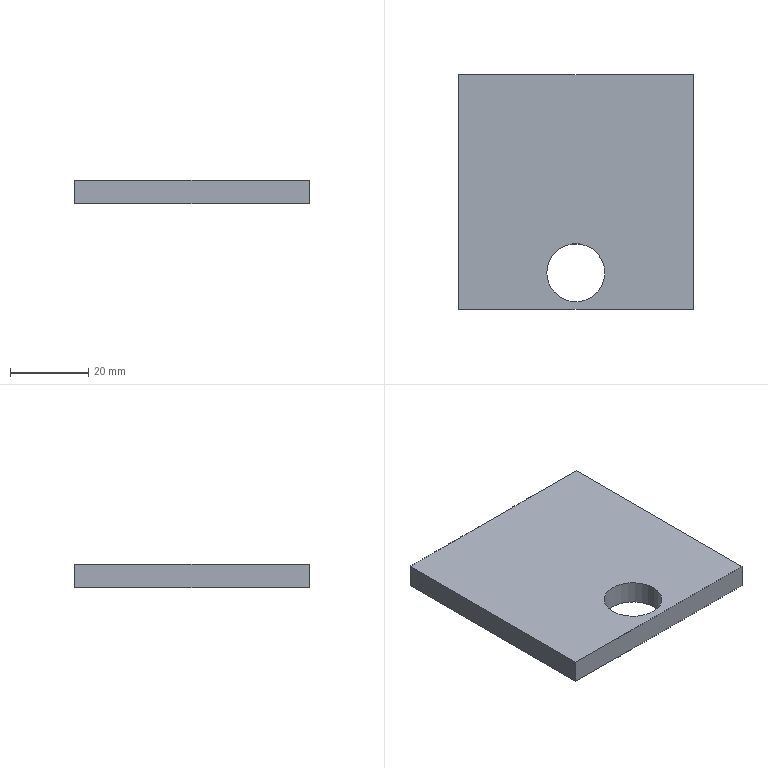Part | NX | features 凸台-拉伸21[4] 2 | 1 solid | 8 faces | box 60 x 60 x 6 mm | volume 20564 mm3 | plane 6 | cylinder 2 | commonest cylinder face diameters 14.829 x2
STEP:
#1=CARTESIAN_POINT('',(2895.533,-50.65,291.015));
#2=VERTEX_POINT('',#1);
#3=CARTESIAN_POINT('',(2895.533,-50.65,297.015));
#4=VERTEX_POINT('',#3);
#5=CARTESIAN_POINT('',(2895.533,-50.65,291.015));
#6=DIRECTION('',(0.,0.,1.));
#7=VECTOR('',#6,1000.);
#8=LINE('',#5,#7);
#9=EDGE_CURVE('',#2,#4,#8,.T.);
#10=ORIENTED_EDGE('',*,*,#9,.F.);
#11=CARTESIAN_POINT('',(2910.361,-50.65,291.015));
#12=VERTEX_POINT('',#11);
#13=CARTESIAN_POINT('',(2902.947,-50.65,291.015));
#14=DIRECTION('',(0.,0.,-1.));
#15=DIRECTION('',(-1.,0.,0.));
#16=AXIS2_PLACEMENT_3D('',#13,#14,#15);
#17=CIRCLE('',#16,7.414);
#18=EDGE_CURVE('',#2,#12,#17,.T.);
#19=ORIENTED_EDGE('',*,*,#18,.T.);
#20=CARTESIAN_POINT('',(2910.361,-50.65,297.015));
#21=VERTEX_POINT('',#20);
#22=CARTESIAN_POINT('',(2910.361,-50.65,291.015));
#23=DIRECTION('',(0.,0.,1.));
#24=VECTOR('',#23,1000.);
#25=LINE('',#22,#24);
#26=EDGE_CURVE('',#21,#12,#25,.F.);
#27=ORIENTED_EDGE('',*,*,#26,.F.);
#28=CARTESIAN_POINT('',(2902.947,-50.65,297.015));
#29=DIRECTION('',(0.,0.,-1.));
#30=DIRECTION('',(-1.,0.,0.));
#31=AXIS2_PLACEMENT_3D('',#28,#29,#30);
#32=CIRCLE('',#31,7.414);
#33=EDGE_CURVE('',#4,#21,#32,.T.);
#34=ORIENTED_EDGE('',*,*,#33,.F.);
#35=EDGE_LOOP('',(#10,#19,#27,#34));
#36=FACE_BOUND('',#35,.T.);
#37=CARTESIAN_POINT('',(2902.947,-50.65,291.015));
#38=DIRECTION('',(0.,0.,1.));
#39=DIRECTION('',(1.,0.,0.));
#40=AXIS2_PLACEMENT_3D('',#37,#38,#39);
#41=CYLINDRICAL_SURFACE('',#40,7.414);
#42=ADVANCED_FACE('',(#36),#41,.F.);
#43=CARTESIAN_POINT('',(2933.,-60.,297.015));
#44=VERTEX_POINT('',#43);
#45=CARTESIAN_POINT('',(2873.,-60.,297.015));
#46=VERTEX_POINT('',#45);
#47=CARTESIAN_POINT('',(2873.,-60.,297.015));
#48=DIRECTION('',(-1.,0.,0.));
#49=VECTOR('',#48,1000.);
#50=LINE('',#47,#49);
#51=EDGE_CURVE('',#44,#46,#50,.T.);
#52=ORIENTED_EDGE('',*,*,#51,.T.);
#53=CARTESIAN_POINT('',(2873.,-60.,291.015));
#54=VERTEX_POINT('',#53);
#55=CARTESIAN_POINT('',(2873.,-60.,291.015));
#56=DIRECTION('',(0.,0.,1.));
#57=VECTOR('',#56,1000.);
#58=LINE('',#55,#57);
#59=EDGE_CURVE('',#54,#46,#58,.T.);
#60=ORIENTED_EDGE('',*,*,#59,.F.);
#61=CARTESIAN_POINT('',(2933.,-60.,291.015));
#62=VERTEX_POINT('',#61);
#63=CARTESIAN_POINT('',(2873.,-60.,291.015));
#64=DIRECTION('',(-1.,0.,0.));
#65=VECTOR('',#64,1000.);
#66=LINE('',#63,#65);
#67=EDGE_CURVE('',#62,#54,#66,.T.);
#68=ORIENTED_EDGE('',*,*,#67,.F.);
#69=CARTESIAN_POINT('',(2933.,-60.,291.015));
#70=DIRECTION('',(0.,0.,1.));
#71=VECTOR('',#70,1000.);
#72=LINE('',#69,#71);
#73=EDGE_CURVE('',#62,#44,#72,.T.);
#74=ORIENTED_EDGE('',*,*,#73,.T.);
#75=EDGE_LOOP('',(#52,#60,#68,#74));
#76=FACE_BOUND('',#75,.T.);
#77=CARTESIAN_POINT('',(2873.,-60.,291.015));
#78=DIRECTION('',(0.,1.,0.));
#79=DIRECTION('',(-1.,0.,0.));
#80=AXIS2_PLACEMENT_3D('',#77,#78,#79);
#81=PLANE('',#80);
#82=ADVANCED_FACE('',(#76),#81,.F.);
#83=CARTESIAN_POINT('',(2933.,0.,297.015));
#84=VERTEX_POINT('',#83);
#85=CARTESIAN_POINT('',(2933.,0.,297.015));
#86=DIRECTION('',(0.,-1.,0.));
#87=VECTOR('',#86,1000.);
#88=LINE('',#85,#87);
#89=EDGE_CURVE('',#84,#44,#88,.T.);
#90=ORIENTED_EDGE('',*,*,#89,.T.);
#91=ORIENTED_EDGE('',*,*,#73,.F.);
#92=CARTESIAN_POINT('',(2933.,0.,291.015));
#93=VERTEX_POINT('',#92);
#94=CARTESIAN_POINT('',(2933.,0.,291.015));
#95=DIRECTION('',(0.,-1.,0.));
#96=VECTOR('',#95,1000.);
#97=LINE('',#94,#96);
#98=EDGE_CURVE('',#93,#62,#97,.T.);
#99=ORIENTED_EDGE('',*,*,#98,.F.);
#100=CARTESIAN_POINT('',(2933.,0.,291.015));
#101=DIRECTION('',(0.,0.,1.));
#102=VECTOR('',#101,1000.);
#103=LINE('',#100,#102);
#104=EDGE_CURVE('',#93,#84,#103,.T.);
#105=ORIENTED_EDGE('',*,*,#104,.T.);
#106=EDGE_LOOP('',(#90,#91,#99,#105));
#107=FACE_BOUND('',#106,.T.);
#108=CARTESIAN_POINT('',(2933.,0.,291.015));
#109=DIRECTION('',(-1.,0.,0.));
#110=DIRECTION('',(0.,-1.,0.));
#111=AXIS2_PLACEMENT_3D('',#108,#109,#110);
#112=PLANE('',#111);
#113=ADVANCED_FACE('',(#107),#112,.F.);
#114=CARTESIAN_POINT('',(2873.,0.,297.015));
#115=VERTEX_POINT('',#114);
#116=CARTESIAN_POINT('',(2873.,0.,297.015));
#117=DIRECTION('',(1.,0.,0.));
#118=VECTOR('',#117,1000.);
#119=LINE('',#116,#118);
#120=EDGE_CURVE('',#115,#84,#119,.T.);
#121=ORIENTED_EDGE('',*,*,#120,.T.);
#122=ORIENTED_EDGE('',*,*,#104,.F.);
#123=CARTESIAN_POINT('',(2873.,0.,291.015));
#124=VERTEX_POINT('',#123);
#125=CARTESIAN_POINT('',(2873.,0.,291.015));
#126=DIRECTION('',(1.,0.,0.));
#127=VECTOR('',#126,1000.);
#128=LINE('',#125,#127);
#129=EDGE_CURVE('',#124,#93,#128,.T.);
#130=ORIENTED_EDGE('',*,*,#129,.F.);
#131=CARTESIAN_POINT('',(2873.,0.,291.015));
#132=DIRECTION('',(0.,0.,1.));
#133=VECTOR('',#132,1000.);
#134=LINE('',#131,#133);
#135=EDGE_CURVE('',#124,#115,#134,.T.);
#136=ORIENTED_EDGE('',*,*,#135,.T.);
#137=EDGE_LOOP('',(#121,#122,#130,#136));
#138=FACE_BOUND('',#137,.T.);
#139=CARTESIAN_POINT('',(2873.,0.,291.015));
#140=DIRECTION('',(0.,-1.,0.));
#141=DIRECTION('',(1.,0.,0.));
#142=AXIS2_PLACEMENT_3D('',#139,#140,#141);
#143=PLANE('',#142);
#144=ADVANCED_FACE('',(#138),#143,.F.);
#145=CARTESIAN_POINT('',(2873.,0.,297.015));
#146=DIRECTION('',(0.,1.,0.));
#147=VECTOR('',#146,1000.);
#148=LINE('',#145,#147);
#149=EDGE_CURVE('',#46,#115,#148,.T.);
#150=ORIENTED_EDGE('',*,*,#149,.T.);
#151=ORIENTED_EDGE('',*,*,#135,.F.);
#152=CARTESIAN_POINT('',(2873.,0.,291.015));
#153=DIRECTION('',(0.,1.,0.));
#154=VECTOR('',#153,1000.);
#155=LINE('',#152,#154);
#156=EDGE_CURVE('',#54,#124,#155,.T.);
#157=ORIENTED_EDGE('',*,*,#156,.F.);
#158=ORIENTED_EDGE('',*,*,#59,.T.);
#159=EDGE_LOOP('',(#150,#151,#157,#158));
#160=FACE_BOUND('',#159,.T.);
#161=CARTESIAN_POINT('',(2873.,0.,291.015));
#162=DIRECTION('',(1.,0.,0.));
#163=DIRECTION('',(0.,0.,-1.));
#164=AXIS2_PLACEMENT_3D('',#161,#162,#163);
#165=PLANE('',#164);
#166=ADVANCED_FACE('',(#160),#165,.F.);
#167=CARTESIAN_POINT('',(2902.947,-50.65,297.015));
#168=DIRECTION('',(0.,0.,-1.));
#169=DIRECTION('',(-1.,0.,0.));
#170=AXIS2_PLACEMENT_3D('',#167,#168,#169);
#171=CIRCLE('',#170,7.414);
#172=EDGE_CURVE('',#21,#4,#171,.T.);
#173=ORIENTED_EDGE('',*,*,#172,.T.);
#174=ORIENTED_EDGE('',*,*,#33,.T.);
#175=EDGE_LOOP('',(#173,#174));
#176=FACE_BOUND('',#175,.T.);
#177=ORIENTED_EDGE('',*,*,#149,.F.);
#178=ORIENTED_EDGE('',*,*,#51,.F.);
#179=ORIENTED_EDGE('',*,*,#89,.F.);
#180=ORIENTED_EDGE('',*,*,#120,.F.);
#181=EDGE_LOOP('',(#177,#178,#179,#180));
#182=FACE_BOUND('',#181,.T.);
#183=CARTESIAN_POINT('',(3000.,0.,297.015));
#184=DIRECTION('',(0.,0.,1.));
#185=DIRECTION('',(1.,0.,0.));
#186=AXIS2_PLACEMENT_3D('',#183,#184,#185);
#187=PLANE('',#186);
#188=ADVANCED_FACE('',(#176,#182),#187,.T.);
#189=CARTESIAN_POINT('',(2902.947,-50.65,291.015));
#190=DIRECTION('',(0.,0.,-1.));
#191=DIRECTION('',(-1.,0.,0.));
#192=AXIS2_PLACEMENT_3D('',#189,#190,#191);
#193=CIRCLE('',#192,7.414);
#194=EDGE_CURVE('',#12,#2,#193,.T.);
#195=ORIENTED_EDGE('',*,*,#194,.F.);
#196=ORIENTED_EDGE('',*,*,#18,.F.);
#197=EDGE_LOOP('',(#195,#196));
#198=FACE_BOUND('',#197,.T.);
#199=ORIENTED_EDGE('',*,*,#156,.T.);
#200=ORIENTED_EDGE('',*,*,#129,.T.);
#201=ORIENTED_EDGE('',*,*,#98,.T.);
#202=ORIENTED_EDGE('',*,*,#67,.T.);
#203=EDGE_LOOP('',(#199,#200,#201,#202));
#204=FACE_BOUND('',#203,.T.);
#205=CARTESIAN_POINT('',(3000.,0.,291.015));
#206=DIRECTION('',(0.,0.,1.));
#207=DIRECTION('',(1.,0.,0.));
#208=AXIS2_PLACEMENT_3D('',#205,#206,#207);
#209=PLANE('',#208);
#210=ADVANCED_FACE('',(#198,#204),#209,.F.);
#211=ORIENTED_EDGE('',*,*,#194,.T.);
#212=ORIENTED_EDGE('',*,*,#9,.T.);
#213=ORIENTED_EDGE('',*,*,#172,.F.);
#214=ORIENTED_EDGE('',*,*,#26,.T.);
#215=EDGE_LOOP('',(#211,#212,#213,#214));
#216=FACE_BOUND('',#215,.T.);
#217=CARTESIAN_POINT('',(2902.947,-50.65,291.015));
#218=DIRECTION('',(0.,0.,1.));
#219=DIRECTION('',(1.,0.,0.));
#220=AXIS2_PLACEMENT_3D('',#217,#218,#219);
#221=CYLINDRICAL_SURFACE('',#220,7.414);
#222=ADVANCED_FACE('',(#216),#221,.F.);
#223=CLOSED_SHELL('',(#42,#82,#113,#144,#166,#188,#210,#222));
#224=MANIFOLD_SOLID_BREP('',#223);
#225=(LENGTH_UNIT()NAMED_UNIT(*)SI_UNIT(.MILLI.,.METRE.));
#226=UNCERTAINTY_MEASURE_WITH_UNIT(LENGTH_MEASURE(0.00001),#225,'','');
#227=(NAMED_UNIT(*)PLANE_ANGLE_UNIT()SI_UNIT($,.RADIAN.));
#228=(NAMED_UNIT(*)SI_UNIT($,.STERADIAN.)SOLID_ANGLE_UNIT());
#229=(GEOMETRIC_REPRESENTATION_CONTEXT(3)GLOBAL_UNCERTAINTY_ASSIGNED_CONTEXT((#226))GLOBAL_UNIT_ASSIGNED_CONTEXT((#225,#227,#228))REPRESENTATION_CONTEXT('',''));
#230=ADVANCED_BREP_SHAPE_REPRESENTATION('',(#224),#229);